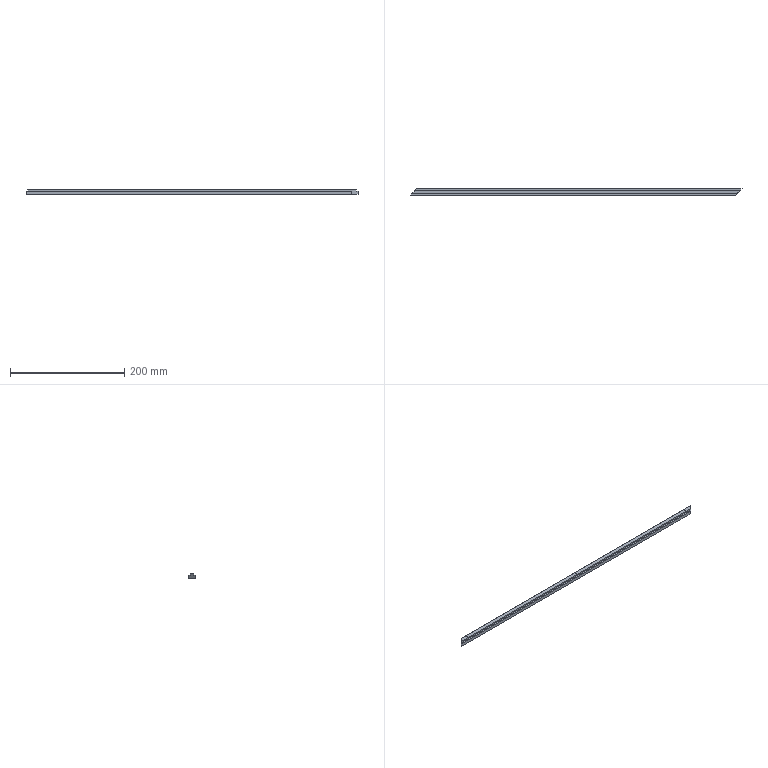Part | STEP file | J013-EBZ05-09-06 | 1 solid | 31 faces | box 581 x 12 x 8 mm | volume 46686 mm3 | plane 13 | cylinder 12 | cone 6 | commonest cylinder face diameters 3.24 x6 4 x6
STEP:
#1=CARTESIAN_POINT('',(285.,6.,7.835));
#2=VERTEX_POINT('',#1);
#3=CARTESIAN_POINT('',(286.62,6.,6.9));
#4=VERTEX_POINT('',#3);
#5=CARTESIAN_POINT('',(286.62,6.,6.9));
#6=DIRECTION('',(0.866,0.,-0.5));
#7=VECTOR('',#6,1000.);
#8=LINE('',#5,#7);
#9=EDGE_CURVE('',#2,#4,#8,.T.);
#10=ORIENTED_EDGE('',*,*,#9,.F.);
#11=CARTESIAN_POINT('',(283.38,6.,6.9));
#12=VERTEX_POINT('',#11);
#13=CARTESIAN_POINT('',(283.38,6.,6.9));
#14=DIRECTION('',(-0.866,0.,-0.5));
#15=VECTOR('',#14,1000.);
#16=LINE('',#13,#15);
#17=EDGE_CURVE('',#2,#12,#16,.T.);
#18=ORIENTED_EDGE('',*,*,#17,.T.);
#19=CARTESIAN_POINT('',(285.,6.,6.9));
#20=DIRECTION('',(0.,0.,-1.));
#21=DIRECTION('',(1.,0.,0.));
#22=AXIS2_PLACEMENT_3D('',#19,#20,#21);
#23=CIRCLE('',#22,1.62);
#24=EDGE_CURVE('',#12,#4,#23,.T.);
#25=ORIENTED_EDGE('',*,*,#24,.T.);
#26=EDGE_LOOP('',(#10,#18,#25));
#27=FACE_OUTER_BOUND('',#26,.T.);
#28=CARTESIAN_POINT('',(285.,6.,6.9));
#29=DIRECTION('',(0.,0.,-1.));
#30=DIRECTION('',(1.,0.,0.));
#31=AXIS2_PLACEMENT_3D('',#28,#29,#30);
#32=CONICAL_SURFACE('',#31,1.62,1.047);
#33=ADVANCED_FACE('',(#27),#32,.F.);
#34=ORIENTED_EDGE('',*,*,#24,.F.);
#35=CARTESIAN_POINT('',(283.38,6.,6.));
#36=VERTEX_POINT('',#35);
#37=CARTESIAN_POINT('',(283.38,6.,0.));
#38=DIRECTION('',(0.,0.,-1.));
#39=VECTOR('',#38,1000.);
#40=LINE('',#37,#39);
#41=EDGE_CURVE('',#12,#36,#40,.T.);
#42=ORIENTED_EDGE('',*,*,#41,.T.);
#43=CARTESIAN_POINT('',(286.62,6.,6.));
#44=VERTEX_POINT('',#43);
#45=CARTESIAN_POINT('',(285.,6.,6.));
#46=DIRECTION('',(0.,0.,-1.));
#47=DIRECTION('',(1.,0.,0.));
#48=AXIS2_PLACEMENT_3D('',#45,#46,#47);
#49=CIRCLE('',#48,1.62);
#50=EDGE_CURVE('',#36,#44,#49,.T.);
#51=ORIENTED_EDGE('',*,*,#50,.T.);
#52=CARTESIAN_POINT('',(286.62,6.,0.));
#53=DIRECTION('',(0.,0.,-1.));
#54=VECTOR('',#53,1000.);
#55=LINE('',#52,#54);
#56=EDGE_CURVE('',#4,#44,#55,.T.);
#57=ORIENTED_EDGE('',*,*,#56,.F.);
#58=EDGE_LOOP('',(#34,#42,#51,#57));
#59=FACE_OUTER_BOUND('',#58,.T.);
#60=CARTESIAN_POINT('',(285.,6.,0.));
#61=DIRECTION('',(0.,0.,-1.));
#62=DIRECTION('',(1.,0.,0.));
#63=AXIS2_PLACEMENT_3D('',#60,#61,#62);
#64=CYLINDRICAL_SURFACE('',#63,1.62);
#65=ADVANCED_FACE('',(#59),#64,.F.);
#66=CARTESIAN_POINT('',(283.,6.,6.));
#67=VERTEX_POINT('',#66);
#68=CARTESIAN_POINT('',(287.,6.,6.));
#69=VERTEX_POINT('',#68);
#70=CARTESIAN_POINT('',(285.,6.,6.));
#71=DIRECTION('',(0.,0.,-1.));
#72=DIRECTION('',(1.,0.,0.));
#73=AXIS2_PLACEMENT_3D('',#70,#71,#72);
#74=CIRCLE('',#73,2.);
#75=EDGE_CURVE('',#67,#69,#74,.T.);
#76=ORIENTED_EDGE('',*,*,#75,.F.);
#77=CARTESIAN_POINT('',(283.,6.,0.));
#78=VERTEX_POINT('',#77);
#79=CARTESIAN_POINT('',(283.,6.,0.));
#80=DIRECTION('',(0.,0.,-1.));
#81=VECTOR('',#80,1000.);
#82=LINE('',#79,#81);
#83=EDGE_CURVE('',#67,#78,#82,.T.);
#84=ORIENTED_EDGE('',*,*,#83,.T.);
#85=CARTESIAN_POINT('',(287.,6.,0.));
#86=VERTEX_POINT('',#85);
#87=CARTESIAN_POINT('',(285.,6.,0.));
#88=DIRECTION('',(0.,0.,-1.));
#89=DIRECTION('',(1.,0.,0.));
#90=AXIS2_PLACEMENT_3D('',#87,#88,#89);
#91=CIRCLE('',#90,2.);
#92=EDGE_CURVE('',#78,#86,#91,.T.);
#93=ORIENTED_EDGE('',*,*,#92,.T.);
#94=CARTESIAN_POINT('',(287.,6.,0.));
#95=DIRECTION('',(0.,0.,-1.));
#96=VECTOR('',#95,1000.);
#97=LINE('',#94,#96);
#98=EDGE_CURVE('',#69,#86,#97,.T.);
#99=ORIENTED_EDGE('',*,*,#98,.F.);
#100=EDGE_LOOP('',(#76,#84,#93,#99));
#101=FACE_OUTER_BOUND('',#100,.T.);
#102=CARTESIAN_POINT('',(285.,6.,0.));
#103=DIRECTION('',(0.,0.,-1.));
#104=DIRECTION('',(1.,0.,0.));
#105=AXIS2_PLACEMENT_3D('',#102,#103,#104);
#106=CYLINDRICAL_SURFACE('',#105,2.);
#107=ADVANCED_FACE('',(#101),#106,.F.);
#108=CARTESIAN_POINT('',(15.,6.,7.835));
#109=VERTEX_POINT('',#108);
#110=CARTESIAN_POINT('',(16.62,6.,6.9));
#111=VERTEX_POINT('',#110);
#112=CARTESIAN_POINT('',(16.62,6.,6.9));
#113=DIRECTION('',(0.866,0.,-0.5));
#114=VECTOR('',#113,1000.);
#115=LINE('',#112,#114);
#116=EDGE_CURVE('',#109,#111,#115,.T.);
#117=ORIENTED_EDGE('',*,*,#116,.F.);
#118=CARTESIAN_POINT('',(13.38,6.,6.9));
#119=VERTEX_POINT('',#118);
#120=CARTESIAN_POINT('',(13.38,6.,6.9));
#121=DIRECTION('',(-0.866,0.,-0.5));
#122=VECTOR('',#121,1000.);
#123=LINE('',#120,#122);
#124=EDGE_CURVE('',#109,#119,#123,.T.);
#125=ORIENTED_EDGE('',*,*,#124,.T.);
#126=CARTESIAN_POINT('',(15.,6.,6.9));
#127=DIRECTION('',(0.,0.,-1.));
#128=DIRECTION('',(1.,0.,0.));
#129=AXIS2_PLACEMENT_3D('',#126,#127,#128);
#130=CIRCLE('',#129,1.62);
#131=EDGE_CURVE('',#119,#111,#130,.T.);
#132=ORIENTED_EDGE('',*,*,#131,.T.);
#133=EDGE_LOOP('',(#117,#125,#132));
#134=FACE_OUTER_BOUND('',#133,.T.);
#135=CARTESIAN_POINT('',(15.,6.,6.9));
#136=DIRECTION('',(0.,0.,-1.));
#137=DIRECTION('',(1.,0.,0.));
#138=AXIS2_PLACEMENT_3D('',#135,#136,#137);
#139=CONICAL_SURFACE('',#138,1.62,1.047);
#140=ADVANCED_FACE('',(#134),#139,.F.);
#141=ORIENTED_EDGE('',*,*,#131,.F.);
#142=CARTESIAN_POINT('',(13.38,6.,6.));
#143=VERTEX_POINT('',#142);
#144=CARTESIAN_POINT('',(13.38,6.,0.));
#145=DIRECTION('',(0.,0.,-1.));
#146=VECTOR('',#145,1000.);
#147=LINE('',#144,#146);
#148=EDGE_CURVE('',#119,#143,#147,.T.);
#149=ORIENTED_EDGE('',*,*,#148,.T.);
#150=CARTESIAN_POINT('',(16.62,6.,6.));
#151=VERTEX_POINT('',#150);
#152=CARTESIAN_POINT('',(15.,6.,6.));
#153=DIRECTION('',(0.,0.,-1.));
#154=DIRECTION('',(1.,0.,0.));
#155=AXIS2_PLACEMENT_3D('',#152,#153,#154);
#156=CIRCLE('',#155,1.62);
#157=EDGE_CURVE('',#143,#151,#156,.T.);
#158=ORIENTED_EDGE('',*,*,#157,.T.);
#159=CARTESIAN_POINT('',(16.62,6.,0.));
#160=DIRECTION('',(0.,0.,-1.));
#161=VECTOR('',#160,1000.);
#162=LINE('',#159,#161);
#163=EDGE_CURVE('',#111,#151,#162,.T.);
#164=ORIENTED_EDGE('',*,*,#163,.F.);
#165=EDGE_LOOP('',(#141,#149,#158,#164));
#166=FACE_OUTER_BOUND('',#165,.T.);
#167=CARTESIAN_POINT('',(15.,6.,0.));
#168=DIRECTION('',(0.,0.,-1.));
#169=DIRECTION('',(1.,0.,0.));
#170=AXIS2_PLACEMENT_3D('',#167,#168,#169);
#171=CYLINDRICAL_SURFACE('',#170,1.62);
#172=ADVANCED_FACE('',(#166),#171,.F.);
#173=CARTESIAN_POINT('',(13.,6.,6.));
#174=VERTEX_POINT('',#173);
#175=CARTESIAN_POINT('',(17.,6.,6.));
#176=VERTEX_POINT('',#175);
#177=CARTESIAN_POINT('',(15.,6.,6.));
#178=DIRECTION('',(0.,0.,-1.));
#179=DIRECTION('',(1.,0.,0.));
#180=AXIS2_PLACEMENT_3D('',#177,#178,#179);
#181=CIRCLE('',#180,2.);
#182=EDGE_CURVE('',#174,#176,#181,.T.);
#183=ORIENTED_EDGE('',*,*,#182,.F.);
#184=CARTESIAN_POINT('',(13.,6.,0.));
#185=VERTEX_POINT('',#184);
#186=CARTESIAN_POINT('',(13.,6.,0.));
#187=DIRECTION('',(0.,0.,-1.));
#188=VECTOR('',#187,1000.);
#189=LINE('',#186,#188);
#190=EDGE_CURVE('',#174,#185,#189,.T.);
#191=ORIENTED_EDGE('',*,*,#190,.T.);
#192=CARTESIAN_POINT('',(17.,6.,0.));
#193=VERTEX_POINT('',#192);
#194=CARTESIAN_POINT('',(15.,6.,0.));
#195=DIRECTION('',(0.,0.,-1.));
#196=DIRECTION('',(1.,0.,0.));
#197=AXIS2_PLACEMENT_3D('',#194,#195,#196);
#198=CIRCLE('',#197,2.);
#199=EDGE_CURVE('',#185,#193,#198,.T.);
#200=ORIENTED_EDGE('',*,*,#199,.T.);
#201=CARTESIAN_POINT('',(17.,6.,0.));
#202=DIRECTION('',(0.,0.,-1.));
#203=VECTOR('',#202,1000.);
#204=LINE('',#201,#203);
#205=EDGE_CURVE('',#176,#193,#204,.T.);
#206=ORIENTED_EDGE('',*,*,#205,.F.);
#207=EDGE_LOOP('',(#183,#191,#200,#206));
#208=FACE_OUTER_BOUND('',#207,.T.);
#209=CARTESIAN_POINT('',(15.,6.,0.));
#210=DIRECTION('',(0.,0.,-1.));
#211=DIRECTION('',(1.,0.,0.));
#212=AXIS2_PLACEMENT_3D('',#209,#210,#211);
#213=CYLINDRICAL_SURFACE('',#212,2.);
#214=ADVANCED_FACE('',(#208),#213,.F.);
#215=CARTESIAN_POINT('',(555.,6.,7.835));
#216=VERTEX_POINT('',#215);
#217=CARTESIAN_POINT('',(556.62,6.,6.9));
#218=VERTEX_POINT('',#217);
#219=CARTESIAN_POINT('',(556.62,6.,6.9));
#220=DIRECTION('',(0.866,0.,-0.5));
#221=VECTOR('',#220,1000.);
#222=LINE('',#219,#221);
#223=EDGE_CURVE('',#216,#218,#222,.T.);
#224=ORIENTED_EDGE('',*,*,#223,.F.);
#225=CARTESIAN_POINT('',(553.38,6.,6.9));
#226=VERTEX_POINT('',#225);
#227=CARTESIAN_POINT('',(553.38,6.,6.9));
#228=DIRECTION('',(-0.866,0.,-0.5));
#229=VECTOR('',#228,1000.);
#230=LINE('',#227,#229);
#231=EDGE_CURVE('',#216,#226,#230,.T.);
#232=ORIENTED_EDGE('',*,*,#231,.T.);
#233=CARTESIAN_POINT('',(555.,6.,6.9));
#234=DIRECTION('',(0.,0.,-1.));
#235=DIRECTION('',(1.,0.,0.));
#236=AXIS2_PLACEMENT_3D('',#233,#234,#235);
#237=CIRCLE('',#236,1.62);
#238=EDGE_CURVE('',#226,#218,#237,.T.);
#239=ORIENTED_EDGE('',*,*,#238,.T.);
#240=EDGE_LOOP('',(#224,#232,#239));
#241=FACE_OUTER_BOUND('',#240,.T.);
#242=CARTESIAN_POINT('',(555.,6.,6.9));
#243=DIRECTION('',(0.,0.,-1.));
#244=DIRECTION('',(1.,0.,0.));
#245=AXIS2_PLACEMENT_3D('',#242,#243,#244);
#246=CONICAL_SURFACE('',#245,1.62,1.047);
#247=ADVANCED_FACE('',(#241),#246,.F.);
#248=ORIENTED_EDGE('',*,*,#238,.F.);
#249=CARTESIAN_POINT('',(553.38,6.,6.));
#250=VERTEX_POINT('',#249);
#251=CARTESIAN_POINT('',(553.38,6.,0.));
#252=DIRECTION('',(0.,0.,-1.));
#253=VECTOR('',#252,1000.);
#254=LINE('',#251,#253);
#255=EDGE_CURVE('',#226,#250,#254,.T.);
#256=ORIENTED_EDGE('',*,*,#255,.T.);
#257=CARTESIAN_POINT('',(556.62,6.,6.));
#258=VERTEX_POINT('',#257);
#259=CARTESIAN_POINT('',(555.,6.,6.));
#260=DIRECTION('',(0.,0.,-1.));
#261=DIRECTION('',(1.,0.,0.));
#262=AXIS2_PLACEMENT_3D('',#259,#260,#261);
#263=CIRCLE('',#262,1.62);
#264=EDGE_CURVE('',#250,#258,#263,.T.);
#265=ORIENTED_EDGE('',*,*,#264,.T.);
#266=CARTESIAN_POINT('',(556.62,6.,0.));
#267=DIRECTION('',(0.,0.,-1.));
#268=VECTOR('',#267,1000.);
#269=LINE('',#266,#268);
#270=EDGE_CURVE('',#218,#258,#269,.T.);
#271=ORIENTED_EDGE('',*,*,#270,.F.);
#272=EDGE_LOOP('',(#248,#256,#265,#271));
#273=FACE_OUTER_BOUND('',#272,.T.);
#274=CARTESIAN_POINT('',(555.,6.,0.));
#275=DIRECTION('',(0.,0.,-1.));
#276=DIRECTION('',(1.,0.,0.));
#277=AXIS2_PLACEMENT_3D('',#274,#275,#276);
#278=CYLINDRICAL_SURFACE('',#277,1.62);
#279=ADVANCED_FACE('',(#273),#278,.F.);
#280=CARTESIAN_POINT('',(553.,6.,6.));
#281=VERTEX_POINT('',#280);
#282=CARTESIAN_POINT('',(557.,6.,6.));
#283=VERTEX_POINT('',#282);
#284=CARTESIAN_POINT('',(555.,6.,6.));
#285=DIRECTION('',(0.,0.,-1.));
#286=DIRECTION('',(1.,0.,0.));
#287=AXIS2_PLACEMENT_3D('',#284,#285,#286);
#288=CIRCLE('',#287,2.);
#289=EDGE_CURVE('',#281,#283,#288,.T.);
#290=ORIENTED_EDGE('',*,*,#289,.F.);
#291=CARTESIAN_POINT('',(553.,6.,0.));
#292=VERTEX_POINT('',#291);
#293=CARTESIAN_POINT('',(553.,6.,0.));
#294=DIRECTION('',(0.,0.,-1.));
#295=VECTOR('',#294,1000.);
#296=LINE('',#293,#295);
#297=EDGE_CURVE('',#281,#292,#296,.T.);
#298=ORIENTED_EDGE('',*,*,#297,.T.);
#299=CARTESIAN_POINT('',(557.,6.,0.));
#300=VERTEX_POINT('',#299);
#301=CARTESIAN_POINT('',(555.,6.,0.));
#302=DIRECTION('',(0.,0.,-1.));
#303=DIRECTION('',(1.,0.,0.));
#304=AXIS2_PLACEMENT_3D('',#301,#302,#303);
#305=CIRCLE('',#304,2.);
#306=EDGE_CURVE('',#292,#300,#305,.T.);
#307=ORIENTED_EDGE('',*,*,#306,.T.);
#308=CARTESIAN_POINT('',(557.,6.,0.));
#309=DIRECTION('',(0.,0.,-1.));
#310=VECTOR('',#309,1000.);
#311=LINE('',#308,#310);
#312=EDGE_CURVE('',#283,#300,#311,.T.);
#313=ORIENTED_EDGE('',*,*,#312,.F.);
#314=EDGE_LOOP('',(#290,#298,#307,#313));
#315=FACE_OUTER_BOUND('',#314,.T.);
#316=CARTESIAN_POINT('',(555.,6.,0.));
#317=DIRECTION('',(0.,0.,-1.));
#318=DIRECTION('',(1.,0.,0.));
#319=AXIS2_PLACEMENT_3D('',#316,#317,#318);
#320=CYLINDRICAL_SURFACE('',#319,2.);
#321=ADVANCED_FACE('',(#315),#320,.F.);
#322=CARTESIAN_POINT('',(6.5,12.,5.5));
#323=VERTEX_POINT('',#322);
#324=CARTESIAN_POINT('',(575.5,12.,5.5));
#325=VERTEX_POINT('',#324);
#326=CARTESIAN_POINT('',(-5.5,12.,5.5));
#327=DIRECTION('',(1.,0.,0.));
#328=VECTOR('',#327,1000.);
#329=LINE('',#326,#328);
#330=EDGE_CURVE('',#323,#325,#329,.T.);
#331=ORIENTED_EDGE('',*,*,#330,.F.);
#332=CARTESIAN_POINT('',(3.8,9.3,5.5));
#333=VERTEX_POINT('',#332);
#334=CARTESIAN_POINT('',(-880.891,-875.391,5.5));
#335=DIRECTION('',(-0.7071,-0.7071,0.));
#336=VECTOR('',#335,1000.);
#337=LINE('',#334,#336);
#338=EDGE_CURVE('',#323,#333,#337,.T.);
#339=ORIENTED_EDGE('',*,*,#338,.T.);
#340=CARTESIAN_POINT('',(572.8,9.3,5.5));
#341=VERTEX_POINT('',#340);
#342=CARTESIAN_POINT('',(-5.5,9.3,5.5));
#343=DIRECTION('',(1.,0.,0.));
#344=VECTOR('',#343,1000.);
#345=LINE('',#342,#344);
#346=EDGE_CURVE('',#333,#341,#345,.T.);
#347=ORIENTED_EDGE('',*,*,#346,.T.);
#348=CARTESIAN_POINT('',(-596.391,-1159.891,5.5));
#349=DIRECTION('',(-0.7071,-0.7071,0.));
#350=VECTOR('',#349,1000.);
#351=LINE('',#348,#350);
#352=EDGE_CURVE('',#325,#341,#351,.T.);
#353=ORIENTED_EDGE('',*,*,#352,.F.);
#354=EDGE_LOOP('',(#331,#339,#347,#353));
#355=FACE_OUTER_BOUND('',#354,.T.);
#356=CARTESIAN_POINT('',(-541.652,-1214.63,5.5));
#357=DIRECTION('',(0.,0.,-1.));
#358=DIRECTION('',(1.,0.,0.));
#359=AXIS2_PLACEMENT_3D('',#356,#357,#358);
#360=PLANE('',#359);
#361=ADVANCED_FACE('',(#355),#360,.F.);
#362=CARTESIAN_POINT('',(563.5,0.,0.));
#363=VERTEX_POINT('',#362);
#364=CARTESIAN_POINT('',(563.5,0.,5.5));
#365=VERTEX_POINT('',#364);
#366=CARTESIAN_POINT('',(563.5,0.,-0.001006));
#367=DIRECTION('',(0.,0.,1.));
#368=VECTOR('',#367,1000.);
#369=LINE('',#366,#368);
#370=EDGE_CURVE('',#363,#365,#369,.T.);
#371=ORIENTED_EDGE('',*,*,#370,.T.);
#372=CARTESIAN_POINT('',(-5.5,0.,5.5));
#373=VERTEX_POINT('',#372);
#374=CARTESIAN_POINT('',(575.5,0.,5.5));
#375=DIRECTION('',(-1.,0.,0.));
#376=VECTOR('',#375,1000.);
#377=LINE('',#374,#376);
#378=EDGE_CURVE('',#365,#373,#377,.T.);
#379=ORIENTED_EDGE('',*,*,#378,.T.);
#380=CARTESIAN_POINT('',(-5.5,0.,0.));
#381=VERTEX_POINT('',#380);
#382=CARTESIAN_POINT('',(-5.5,0.,0.));
#383=DIRECTION('',(0.,0.,1.));
#384=VECTOR('',#383,1000.);
#385=LINE('',#382,#384);
#386=EDGE_CURVE('',#381,#373,#385,.T.);
#387=ORIENTED_EDGE('',*,*,#386,.F.);
#388=CARTESIAN_POINT('',(575.5,0.,0.));
#389=DIRECTION('',(-1.,0.,0.));
#390=VECTOR('',#389,1000.);
#391=LINE('',#388,#390);
#392=EDGE_CURVE('',#363,#381,#391,.T.);
#393=ORIENTED_EDGE('',*,*,#392,.F.);
#394=EDGE_LOOP('',(#371,#379,#387,#393));
#395=FACE_OUTER_BOUND('',#394,.T.);
#396=CARTESIAN_POINT('',(575.5,0.,0.));
#397=DIRECTION('',(0.,1.,0.));
#398=DIRECTION('',(0.,0.,1.));
#399=AXIS2_PLACEMENT_3D('',#396,#397,#398);
#400=PLANE('',#399);
#401=ADVANCED_FACE('',(#395),#400,.F.);
#402=CARTESIAN_POINT('',(6.5,12.,0.));
#403=VERTEX_POINT('',#402);
#404=CARTESIAN_POINT('',(-880.891,-875.391,0.));
#405=DIRECTION('',(-0.7071,-0.7071,0.));
#406=VECTOR('',#405,1000.);
#407=LINE('',#404,#406);
#408=EDGE_CURVE('',#403,#381,#407,.T.);
#409=ORIENTED_EDGE('',*,*,#408,.F.);
#410=CARTESIAN_POINT('',(575.5,12.,0.));
#411=VERTEX_POINT('',#410);
#412=CARTESIAN_POINT('',(-5.5,12.,0.));
#413=DIRECTION('',(1.,0.,0.));
#414=VECTOR('',#413,1000.);
#415=LINE('',#412,#414);
#416=EDGE_CURVE('',#403,#411,#415,.T.);
#417=ORIENTED_EDGE('',*,*,#416,.T.);
#418=CARTESIAN_POINT('',(-596.391,-1159.891,0.));
#419=DIRECTION('',(-0.7071,-0.7071,0.));
#420=VECTOR('',#419,1000.);
#421=LINE('',#418,#420);
#422=EDGE_CURVE('',#411,#363,#421,.T.);
#423=ORIENTED_EDGE('',*,*,#422,.T.);
#424=ORIENTED_EDGE('',*,*,#392,.T.);
#425=EDGE_LOOP('',(#409,#417,#423,#424));
#426=FACE_OUTER_BOUND('',#425,.T.);
#427=CARTESIAN_POINT('',(285.,6.,0.));
#428=DIRECTION('',(0.,0.,-1.));
#429=DIRECTION('',(1.,0.,0.));
#430=AXIS2_PLACEMENT_3D('',#427,#428,#429);
#431=CIRCLE('',#430,2.);
#432=EDGE_CURVE('',#86,#78,#431,.T.);
#433=ORIENTED_EDGE('',*,*,#432,.F.);
#434=ORIENTED_EDGE('',*,*,#92,.F.);
#435=EDGE_LOOP('',(#433,#434));
#436=FACE_BOUND('',#435,.T.);
#437=CARTESIAN_POINT('',(15.,6.,0.));
#438=DIRECTION('',(0.,0.,-1.));
#439=DIRECTION('',(1.,0.,0.));
#440=AXIS2_PLACEMENT_3D('',#437,#438,#439);
#441=CIRCLE('',#440,2.);
#442=EDGE_CURVE('',#193,#185,#441,.T.);
#443=ORIENTED_EDGE('',*,*,#442,.F.);
#444=ORIENTED_EDGE('',*,*,#199,.F.);
#445=EDGE_LOOP('',(#443,#444));
#446=FACE_BOUND('',#445,.T.);
#447=CARTESIAN_POINT('',(555.,6.,0.));
#448=DIRECTION('',(0.,0.,-1.));
#449=DIRECTION('',(1.,0.,0.));
#450=AXIS2_PLACEMENT_3D('',#447,#448,#449);
#451=CIRCLE('',#450,2.);
#452=EDGE_CURVE('',#300,#292,#451,.T.);
#453=ORIENTED_EDGE('',*,*,#452,.F.);
#454=ORIENTED_EDGE('',*,*,#306,.F.);
#455=EDGE_LOOP('',(#453,#454));
#456=FACE_BOUND('',#455,.T.);
#457=CARTESIAN_POINT('',(-541.652,-1214.63,0.));
#458=DIRECTION('',(0.,0.,-1.));
#459=DIRECTION('',(1.,0.,0.));
#460=AXIS2_PLACEMENT_3D('',#457,#458,#459);
#461=PLANE('',#460);
#462=ADVANCED_FACE('',(#426,#436,#446,#456),#461,.T.);
#463=CARTESIAN_POINT('',(566.2,2.7,5.5));
#464=VERTEX_POINT('',#463);
#465=CARTESIAN_POINT('',(-2.8,2.7,5.5));
#466=VERTEX_POINT('',#465);
#467=CARTESIAN_POINT('',(575.5,2.7,5.5));
#468=DIRECTION('',(-1.,0.,0.));
#469=VECTOR('',#468,1000.);
#470=LINE('',#467,#469);
#471=EDGE_CURVE('',#464,#466,#470,.T.);
#472=ORIENTED_EDGE('',*,*,#471,.T.);
#473=CARTESIAN_POINT('',(-880.891,-875.391,5.5));
#474=DIRECTION('',(-0.7071,-0.7071,0.));
#475=VECTOR('',#474,1000.);
#476=LINE('',#473,#475);
#477=EDGE_CURVE('',#466,#373,#476,.T.);
#478=ORIENTED_EDGE('',*,*,#477,.T.);
#479=ORIENTED_EDGE('',*,*,#378,.F.);
#480=CARTESIAN_POINT('',(-596.391,-1159.891,5.5));
#481=DIRECTION('',(-0.7071,-0.7071,0.));
#482=VECTOR('',#481,1000.);
#483=LINE('',#480,#482);
#484=EDGE_CURVE('',#464,#365,#483,.T.);
#485=ORIENTED_EDGE('',*,*,#484,.F.);
#486=EDGE_LOOP('',(#472,#478,#479,#485));
#487=FACE_OUTER_BOUND('',#486,.T.);
#488=CARTESIAN_POINT('',(-541.652,-1214.63,5.5));
#489=DIRECTION('',(0.,0.,-1.));
#490=DIRECTION('',(1.,0.,0.));
#491=AXIS2_PLACEMENT_3D('',#488,#489,#490);
#492=PLANE('',#491);
#493=ADVANCED_FACE('',(#487),#492,.F.);
#494=CARTESIAN_POINT('',(3.8,9.3,8.));
#495=VERTEX_POINT('',#494);
#496=CARTESIAN_POINT('',(3.8,9.3,8.));
#497=DIRECTION('',(0.,0.,-1.));
#498=VECTOR('',#497,1000.);
#499=LINE('',#496,#498);
#500=EDGE_CURVE('',#495,#333,#499,.T.);
#501=ORIENTED_EDGE('',*,*,#500,.F.);
#502=CARTESIAN_POINT('',(572.8,9.3,8.));
#503=VERTEX_POINT('',#502);
#504=CARTESIAN_POINT('',(-5.5,9.3,8.));
#505=DIRECTION('',(1.,0.,0.));
#506=VECTOR('',#505,1000.);
#507=LINE('',#504,#506);
#508=EDGE_CURVE('',#495,#503,#507,.T.);
#509=ORIENTED_EDGE('',*,*,#508,.T.);
#510=CARTESIAN_POINT('',(572.8,9.3,8.));
#511=DIRECTION('',(0.,0.,-1.));
#512=VECTOR('',#511,1000.);
#513=LINE('',#510,#512);
#514=EDGE_CURVE('',#503,#341,#513,.T.);
#515=ORIENTED_EDGE('',*,*,#514,.T.);
#516=ORIENTED_EDGE('',*,*,#346,.F.);
#517=EDGE_LOOP('',(#501,#509,#515,#516));
#518=FACE_OUTER_BOUND('',#517,.T.);
#519=CARTESIAN_POINT('',(-5.5,9.3,8.));
#520=DIRECTION('',(0.,1.,0.));
#521=DIRECTION('',(0.,0.,1.));
#522=AXIS2_PLACEMENT_3D('',#519,#520,#521);
#523=PLANE('',#522);
#524=ADVANCED_FACE('',(#518),#523,.T.);
#525=CARTESIAN_POINT('',(-2.8,2.7,8.));
#526=VERTEX_POINT('',#525);
#527=CARTESIAN_POINT('',(-2.8,2.7,8.));
#528=DIRECTION('',(0.,0.,1.));
#529=VECTOR('',#528,1000.);
#530=LINE('',#527,#529);
#531=EDGE_CURVE('',#466,#526,#530,.T.);
#532=ORIENTED_EDGE('',*,*,#531,.F.);
#533=ORIENTED_EDGE('',*,*,#471,.F.);
#534=CARTESIAN_POINT('',(566.2,2.7,8.));
#535=VERTEX_POINT('',#534);
#536=CARTESIAN_POINT('',(566.2,2.7,8.));
#537=DIRECTION('',(0.,0.,1.));
#538=VECTOR('',#537,1000.);
#539=LINE('',#536,#538);
#540=EDGE_CURVE('',#464,#535,#539,.T.);
#541=ORIENTED_EDGE('',*,*,#540,.T.);
#542=CARTESIAN_POINT('',(575.5,2.7,8.));
#543=DIRECTION('',(-1.,0.,0.));
#544=VECTOR('',#543,1000.);
#545=LINE('',#542,#544);
#546=EDGE_CURVE('',#535,#526,#545,.T.);
#547=ORIENTED_EDGE('',*,*,#546,.T.);
#548=EDGE_LOOP('',(#532,#533,#541,#547));
#549=FACE_OUTER_BOUND('',#548,.T.);
#550=CARTESIAN_POINT('',(575.5,2.7,8.));
#551=DIRECTION('',(0.,-1.,0.));
#552=DIRECTION('',(0.,0.,-1.));
#553=AXIS2_PLACEMENT_3D('',#550,#551,#552);
#554=PLANE('',#553);
#555=ADVANCED_FACE('',(#549),#554,.T.);
#556=ORIENTED_EDGE('',*,*,#508,.F.);
#557=CARTESIAN_POINT('',(-880.891,-875.391,8.));
#558=DIRECTION('',(-0.7071,-0.7071,0.));
#559=VECTOR('',#558,1000.);
#560=LINE('',#557,#559);
#561=EDGE_CURVE('',#495,#526,#560,.T.);
#562=ORIENTED_EDGE('',*,*,#561,.T.);
#563=ORIENTED_EDGE('',*,*,#546,.F.);
#564=CARTESIAN_POINT('',(-596.391,-1159.891,8.));
#565=DIRECTION('',(-0.7071,-0.7071,0.));
#566=VECTOR('',#565,1000.);
#567=LINE('',#564,#566);
#568=EDGE_CURVE('',#503,#535,#567,.T.);
#569=ORIENTED_EDGE('',*,*,#568,.F.);
#570=EDGE_LOOP('',(#556,#562,#563,#569));
#571=FACE_OUTER_BOUND('',#570,.T.);
#572=CARTESIAN_POINT('',(-541.652,-1214.629,8.));
#573=DIRECTION('',(0.,0.,-1.));
#574=DIRECTION('',(1.,0.,0.));
#575=AXIS2_PLACEMENT_3D('',#572,#573,#574);
#576=PLANE('',#575);
#577=ADVANCED_FACE('',(#571),#576,.F.);
#578=ORIENTED_EDGE('',*,*,#416,.F.);
#579=CARTESIAN_POINT('',(6.5,12.,-0.001006));
#580=DIRECTION('',(0.,0.,1.));
#581=VECTOR('',#580,1000.);
#582=LINE('',#579,#581);
#583=EDGE_CURVE('',#403,#323,#582,.T.);
#584=ORIENTED_EDGE('',*,*,#583,.T.);
#585=ORIENTED_EDGE('',*,*,#330,.T.);
#586=CARTESIAN_POINT('',(575.5,12.,0.));
#587=DIRECTION('',(0.,0.,1.));
#588=VECTOR('',#587,1000.);
#589=LINE('',#586,#588);
#590=EDGE_CURVE('',#411,#325,#589,.T.);
#591=ORIENTED_EDGE('',*,*,#590,.F.);
#592=EDGE_LOOP('',(#578,#584,#585,#591));
#593=FACE_OUTER_BOUND('',#592,.T.);
#594=CARTESIAN_POINT('',(-5.5,12.,0.));
#595=DIRECTION('',(0.,-1.,0.));
#596=DIRECTION('',(0.,0.,-1.));
#597=AXIS2_PLACEMENT_3D('',#594,#595,#596);
#598=PLANE('',#597);
#599=ADVANCED_FACE('',(#593),#598,.F.);
#600=ORIENTED_EDGE('',*,*,#297,.F.);
#601=CARTESIAN_POINT('',(555.,6.,6.));
#602=DIRECTION('',(0.,0.,-1.));
#603=DIRECTION('',(1.,0.,0.));
#604=AXIS2_PLACEMENT_3D('',#601,#602,#603);
#605=CIRCLE('',#604,2.);
#606=EDGE_CURVE('',#283,#281,#605,.T.);
#607=ORIENTED_EDGE('',*,*,#606,.F.);
#608=ORIENTED_EDGE('',*,*,#312,.T.);
#609=ORIENTED_EDGE('',*,*,#452,.T.);
#610=EDGE_LOOP('',(#600,#607,#608,#609));
#611=FACE_OUTER_BOUND('',#610,.T.);
#612=CARTESIAN_POINT('',(555.,6.,0.));
#613=DIRECTION('',(0.,0.,-1.));
#614=DIRECTION('',(1.,0.,0.));
#615=AXIS2_PLACEMENT_3D('',#612,#613,#614);
#616=CYLINDRICAL_SURFACE('',#615,2.);
#617=ADVANCED_FACE('',(#611),#616,.F.);
#618=CARTESIAN_POINT('',(555.,6.,6.));
#619=DIRECTION('',(0.,0.,-1.));
#620=DIRECTION('',(1.,0.,0.));
#621=AXIS2_PLACEMENT_3D('',#618,#619,#620);
#622=CIRCLE('',#621,1.62);
#623=EDGE_CURVE('',#258,#250,#622,.T.);
#624=ORIENTED_EDGE('',*,*,#623,.F.);
#625=ORIENTED_EDGE('',*,*,#264,.F.);
#626=EDGE_LOOP('',(#624,#625));
#627=FACE_BOUND('',#626,.T.);
#628=ORIENTED_EDGE('',*,*,#606,.T.);
#629=ORIENTED_EDGE('',*,*,#289,.T.);
#630=EDGE_LOOP('',(#628,#629));
#631=FACE_OUTER_BOUND('',#630,.T.);
#632=CARTESIAN_POINT('',(553.,6.,6.));
#633=DIRECTION('',(0.,0.,1.));
#634=DIRECTION('',(-1.,0.,0.));
#635=AXIS2_PLACEMENT_3D('',#632,#633,#634);
#636=PLANE('',#635);
#637=ADVANCED_FACE('',(#627,#631),#636,.F.);
#638=ORIENTED_EDGE('',*,*,#255,.F.);
#639=CARTESIAN_POINT('',(555.,6.,6.9));
#640=DIRECTION('',(0.,0.,-1.));
#641=DIRECTION('',(1.,0.,0.));
#642=AXIS2_PLACEMENT_3D('',#639,#640,#641);
#643=CIRCLE('',#642,1.62);
#644=EDGE_CURVE('',#218,#226,#643,.T.);
#645=ORIENTED_EDGE('',*,*,#644,.F.);
#646=ORIENTED_EDGE('',*,*,#270,.T.);
#647=ORIENTED_EDGE('',*,*,#623,.T.);
#648=EDGE_LOOP('',(#638,#645,#646,#647));
#649=FACE_OUTER_BOUND('',#648,.T.);
#650=CARTESIAN_POINT('',(555.,6.,0.));
#651=DIRECTION('',(0.,0.,-1.));
#652=DIRECTION('',(1.,0.,0.));
#653=AXIS2_PLACEMENT_3D('',#650,#651,#652);
#654=CYLINDRICAL_SURFACE('',#653,1.62);
#655=ADVANCED_FACE('',(#649),#654,.F.);
#656=ORIENTED_EDGE('',*,*,#231,.F.);
#657=ORIENTED_EDGE('',*,*,#223,.T.);
#658=ORIENTED_EDGE('',*,*,#644,.T.);
#659=EDGE_LOOP('',(#656,#657,#658));
#660=FACE_OUTER_BOUND('',#659,.T.);
#661=CARTESIAN_POINT('',(555.,6.,6.9));
#662=DIRECTION('',(0.,0.,-1.));
#663=DIRECTION('',(1.,0.,0.));
#664=AXIS2_PLACEMENT_3D('',#661,#662,#663);
#665=CONICAL_SURFACE('',#664,1.62,1.047);
#666=ADVANCED_FACE('',(#660),#665,.F.);
#667=ORIENTED_EDGE('',*,*,#190,.F.);
#668=CARTESIAN_POINT('',(15.,6.,6.));
#669=DIRECTION('',(0.,0.,-1.));
#670=DIRECTION('',(1.,0.,0.));
#671=AXIS2_PLACEMENT_3D('',#668,#669,#670);
#672=CIRCLE('',#671,2.);
#673=EDGE_CURVE('',#176,#174,#672,.T.);
#674=ORIENTED_EDGE('',*,*,#673,.F.);
#675=ORIENTED_EDGE('',*,*,#205,.T.);
#676=ORIENTED_EDGE('',*,*,#442,.T.);
#677=EDGE_LOOP('',(#667,#674,#675,#676));
#678=FACE_OUTER_BOUND('',#677,.T.);
#679=CARTESIAN_POINT('',(15.,6.,0.));
#680=DIRECTION('',(0.,0.,-1.));
#681=DIRECTION('',(1.,0.,0.));
#682=AXIS2_PLACEMENT_3D('',#679,#680,#681);
#683=CYLINDRICAL_SURFACE('',#682,2.);
#684=ADVANCED_FACE('',(#678),#683,.F.);
#685=CARTESIAN_POINT('',(15.,6.,6.));
#686=DIRECTION('',(0.,0.,-1.));
#687=DIRECTION('',(1.,0.,0.));
#688=AXIS2_PLACEMENT_3D('',#685,#686,#687);
#689=CIRCLE('',#688,1.62);
#690=EDGE_CURVE('',#151,#143,#689,.T.);
#691=ORIENTED_EDGE('',*,*,#690,.F.);
#692=ORIENTED_EDGE('',*,*,#157,.F.);
#693=EDGE_LOOP('',(#691,#692));
#694=FACE_BOUND('',#693,.T.);
#695=ORIENTED_EDGE('',*,*,#673,.T.);
#696=ORIENTED_EDGE('',*,*,#182,.T.);
#697=EDGE_LOOP('',(#695,#696));
#698=FACE_OUTER_BOUND('',#697,.T.);
#699=CARTESIAN_POINT('',(13.,6.,6.));
#700=DIRECTION('',(0.,0.,1.));
#701=DIRECTION('',(-1.,0.,0.));
#702=AXIS2_PLACEMENT_3D('',#699,#700,#701);
#703=PLANE('',#702);
#704=ADVANCED_FACE('',(#694,#698),#703,.F.);
#705=ORIENTED_EDGE('',*,*,#148,.F.);
#706=CARTESIAN_POINT('',(15.,6.,6.9));
#707=DIRECTION('',(0.,0.,-1.));
#708=DIRECTION('',(1.,0.,0.));
#709=AXIS2_PLACEMENT_3D('',#706,#707,#708);
#710=CIRCLE('',#709,1.62);
#711=EDGE_CURVE('',#111,#119,#710,.T.);
#712=ORIENTED_EDGE('',*,*,#711,.F.);
#713=ORIENTED_EDGE('',*,*,#163,.T.);
#714=ORIENTED_EDGE('',*,*,#690,.T.);
#715=EDGE_LOOP('',(#705,#712,#713,#714));
#716=FACE_OUTER_BOUND('',#715,.T.);
#717=CARTESIAN_POINT('',(15.,6.,0.));
#718=DIRECTION('',(0.,0.,-1.));
#719=DIRECTION('',(1.,0.,0.));
#720=AXIS2_PLACEMENT_3D('',#717,#718,#719);
#721=CYLINDRICAL_SURFACE('',#720,1.62);
#722=ADVANCED_FACE('',(#716),#721,.F.);
#723=ORIENTED_EDGE('',*,*,#124,.F.);
#724=ORIENTED_EDGE('',*,*,#116,.T.);
#725=ORIENTED_EDGE('',*,*,#711,.T.);
#726=EDGE_LOOP('',(#723,#724,#725));
#727=FACE_OUTER_BOUND('',#726,.T.);
#728=CARTESIAN_POINT('',(15.,6.,6.9));
#729=DIRECTION('',(0.,0.,-1.));
#730=DIRECTION('',(1.,0.,0.));
#731=AXIS2_PLACEMENT_3D('',#728,#729,#730);
#732=CONICAL_SURFACE('',#731,1.62,1.047);
#733=ADVANCED_FACE('',(#727),#732,.F.);
#734=ORIENTED_EDGE('',*,*,#83,.F.);
#735=CARTESIAN_POINT('',(285.,6.,6.));
#736=DIRECTION('',(0.,0.,-1.));
#737=DIRECTION('',(1.,0.,0.));
#738=AXIS2_PLACEMENT_3D('',#735,#736,#737);
#739=CIRCLE('',#738,2.);
#740=EDGE_CURVE('',#69,#67,#739,.T.);
#741=ORIENTED_EDGE('',*,*,#740,.F.);
#742=ORIENTED_EDGE('',*,*,#98,.T.);
#743=ORIENTED_EDGE('',*,*,#432,.T.);
#744=EDGE_LOOP('',(#734,#741,#742,#743));
#745=FACE_OUTER_BOUND('',#744,.T.);
#746=CARTESIAN_POINT('',(285.,6.,0.));
#747=DIRECTION('',(0.,0.,-1.));
#748=DIRECTION('',(1.,0.,0.));
#749=AXIS2_PLACEMENT_3D('',#746,#747,#748);
#750=CYLINDRICAL_SURFACE('',#749,2.);
#751=ADVANCED_FACE('',(#745),#750,.F.);
#752=CARTESIAN_POINT('',(285.,6.,6.));
#753=DIRECTION('',(0.,0.,-1.));
#754=DIRECTION('',(1.,0.,0.));
#755=AXIS2_PLACEMENT_3D('',#752,#753,#754);
#756=CIRCLE('',#755,1.62);
#757=EDGE_CURVE('',#44,#36,#756,.T.);
#758=ORIENTED_EDGE('',*,*,#757,.F.);
#759=ORIENTED_EDGE('',*,*,#50,.F.);
#760=EDGE_LOOP('',(#758,#759));
#761=FACE_BOUND('',#760,.T.);
#762=ORIENTED_EDGE('',*,*,#740,.T.);
#763=ORIENTED_EDGE('',*,*,#75,.T.);
#764=EDGE_LOOP('',(#762,#763));
#765=FACE_OUTER_BOUND('',#764,.T.);
#766=CARTESIAN_POINT('',(283.,6.,6.));
#767=DIRECTION('',(0.,0.,1.));
#768=DIRECTION('',(-1.,0.,0.));
#769=AXIS2_PLACEMENT_3D('',#766,#767,#768);
#770=PLANE('',#769);
#771=ADVANCED_FACE('',(#761,#765),#770,.F.);
#772=ORIENTED_EDGE('',*,*,#41,.F.);
#773=CARTESIAN_POINT('',(285.,6.,6.9));
#774=DIRECTION('',(0.,0.,-1.));
#775=DIRECTION('',(1.,0.,0.));
#776=AXIS2_PLACEMENT_3D('',#773,#774,#775);
#777=CIRCLE('',#776,1.62);
#778=EDGE_CURVE('',#4,#12,#777,.T.);
#779=ORIENTED_EDGE('',*,*,#778,.F.);
#780=ORIENTED_EDGE('',*,*,#56,.T.);
#781=ORIENTED_EDGE('',*,*,#757,.T.);
#782=EDGE_LOOP('',(#772,#779,#780,#781));
#783=FACE_OUTER_BOUND('',#782,.T.);
#784=CARTESIAN_POINT('',(285.,6.,0.));
#785=DIRECTION('',(0.,0.,-1.));
#786=DIRECTION('',(1.,0.,0.));
#787=AXIS2_PLACEMENT_3D('',#784,#785,#786);
#788=CYLINDRICAL_SURFACE('',#787,1.62);
#789=ADVANCED_FACE('',(#783),#788,.F.);
#790=ORIENTED_EDGE('',*,*,#17,.F.);
#791=ORIENTED_EDGE('',*,*,#9,.T.);
#792=ORIENTED_EDGE('',*,*,#778,.T.);
#793=EDGE_LOOP('',(#790,#791,#792));
#794=FACE_OUTER_BOUND('',#793,.T.);
#795=CARTESIAN_POINT('',(285.,6.,6.9));
#796=DIRECTION('',(0.,0.,-1.));
#797=DIRECTION('',(1.,0.,0.));
#798=AXIS2_PLACEMENT_3D('',#795,#796,#797);
#799=CONICAL_SURFACE('',#798,1.62,1.047);
#800=ADVANCED_FACE('',(#794),#799,.F.);
#801=ORIENTED_EDGE('',*,*,#422,.F.);
#802=ORIENTED_EDGE('',*,*,#590,.T.);
#803=ORIENTED_EDGE('',*,*,#352,.T.);
#804=ORIENTED_EDGE('',*,*,#514,.F.);
#805=ORIENTED_EDGE('',*,*,#568,.T.);
#806=ORIENTED_EDGE('',*,*,#540,.F.);
#807=ORIENTED_EDGE('',*,*,#484,.T.);
#808=ORIENTED_EDGE('',*,*,#370,.F.);
#809=EDGE_LOOP('',(#801,#802,#803,#804,#805,#806,#807,#808));
#810=FACE_OUTER_BOUND('',#809,.T.);
#811=CARTESIAN_POINT('',(563.5,0.,-0.001006));
#812=DIRECTION('',(0.7071,-0.7071,0.));
#813=DIRECTION('',(0.7071,0.7071,0.));
#814=AXIS2_PLACEMENT_3D('',#811,#812,#813);
#815=PLANE('',#814);
#816=ADVANCED_FACE('',(#810),#815,.T.);
#817=ORIENTED_EDGE('',*,*,#583,.F.);
#818=ORIENTED_EDGE('',*,*,#408,.T.);
#819=ORIENTED_EDGE('',*,*,#386,.T.);
#820=ORIENTED_EDGE('',*,*,#477,.F.);
#821=ORIENTED_EDGE('',*,*,#531,.T.);
#822=ORIENTED_EDGE('',*,*,#561,.F.);
#823=ORIENTED_EDGE('',*,*,#500,.T.);
#824=ORIENTED_EDGE('',*,*,#338,.F.);
#825=EDGE_LOOP('',(#817,#818,#819,#820,#821,#822,#823,#824));
#826=FACE_OUTER_BOUND('',#825,.T.);
#827=CARTESIAN_POINT('',(-5.5,0.,-0.001006));
#828=DIRECTION('',(0.7071,-0.7071,0.));
#829=DIRECTION('',(0.7071,0.7071,0.));
#830=AXIS2_PLACEMENT_3D('',#827,#828,#829);
#831=PLANE('',#830);
#832=ADVANCED_FACE('',(#826),#831,.F.);
#833=CLOSED_SHELL('',(#33,#65,#107,#140,#172,#214,#247,#279,#321,#361,#401,#462,#493,#524,#555,#577,#599,#617,#637,#655,#666,#684,#704,#722,#733,#751,#771,#789,#800,#816,#832));
#834=MANIFOLD_SOLID_BREP('',#833);
#835=CARTESIAN_POINT('',(0.,0.,0.));
#836=DIRECTION('',(0.,0.,1.));
#837=DIRECTION('',(1.,0.,0.));
#838=AXIS2_PLACEMENT_3D('',#835,#836,#837);
#839=(LENGTH_UNIT()NAMED_UNIT(*)SI_UNIT(.MILLI.,.METRE.));
#840=UNCERTAINTY_MEASURE_WITH_UNIT(LENGTH_MEASURE(0.00001),#839,'','');
#841=(NAMED_UNIT(*)PLANE_ANGLE_UNIT()SI_UNIT($,.RADIAN.));
#842=(NAMED_UNIT(*)SI_UNIT($,.STERADIAN.)SOLID_ANGLE_UNIT());
#843=(GEOMETRIC_REPRESENTATION_CONTEXT(3)GLOBAL_UNCERTAINTY_ASSIGNED_CONTEXT((#840))GLOBAL_UNIT_ASSIGNED_CONTEXT((#839,#841,#842))REPRESENTATION_CONTEXT('',''));
#844=ADVANCED_BREP_SHAPE_REPRESENTATION('',(#834,#838),#843);